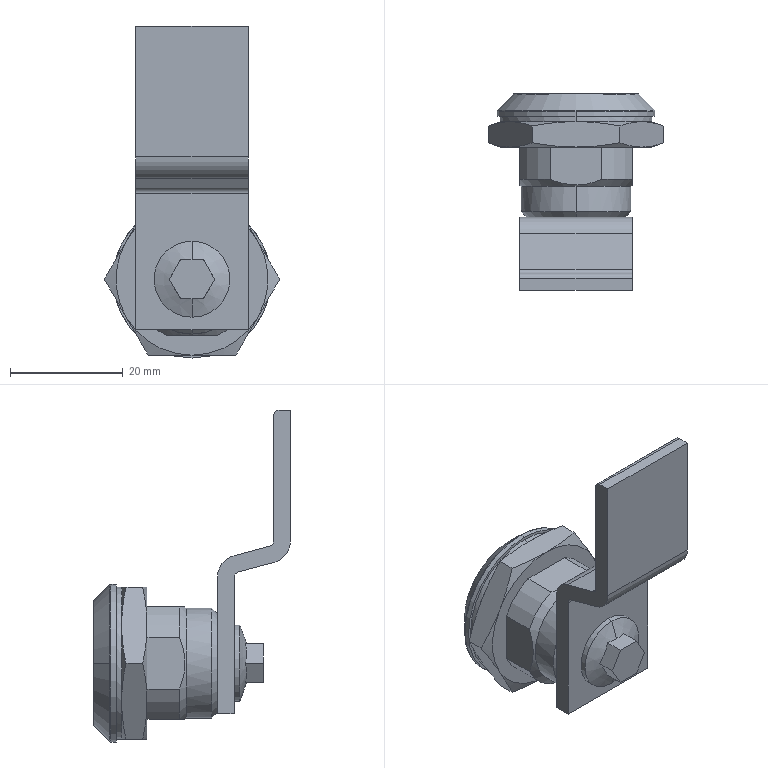Part | SolidWorks | features BaseBody 1 | 1 solid | 81 faces | box 31.177 x 35 x 59 mm | volume 12779 mm3 | plane 35 | cylinder 22 | cone 20 | spline 4 | commonest cylinder face diameters 22 x4 2 x3 9.2 x3 8 x2 13.5 x2 15.8 x2